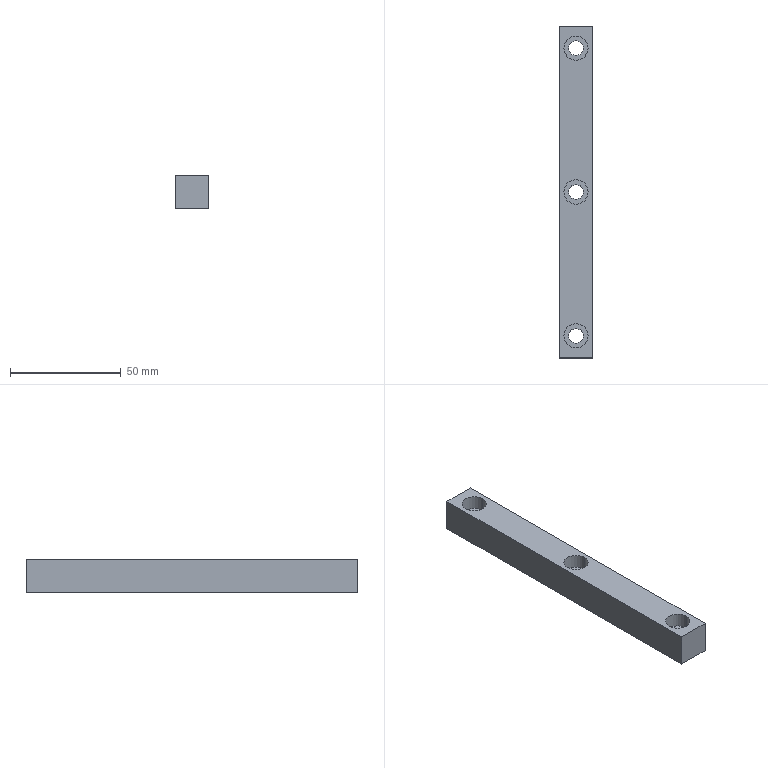Part | STEP file | BASE.STOPPER.stp | 1 solid | 21 faces | box 15 x 150 x 15 mm | volume 31025 mm3 | cylinder 8 | plane 7 | spline 6 | commonest cylinder face diameters 6.6 x4 11 x4